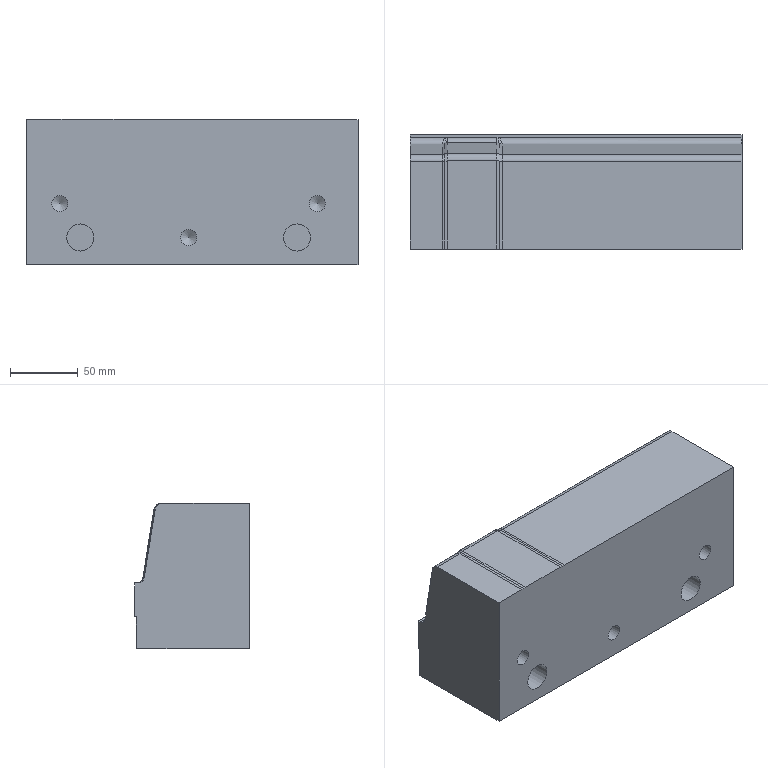Part | NX | features solid 2 | 1 solid | 51 faces | box 245 x 84.473 x 107.229 mm | volume 2020189 mm3 | spline 19 | cylinder 15 | plane 14 | cone 3 | commonest cylinder face diameters 8 x5 10 x5 12 x3 20 x2